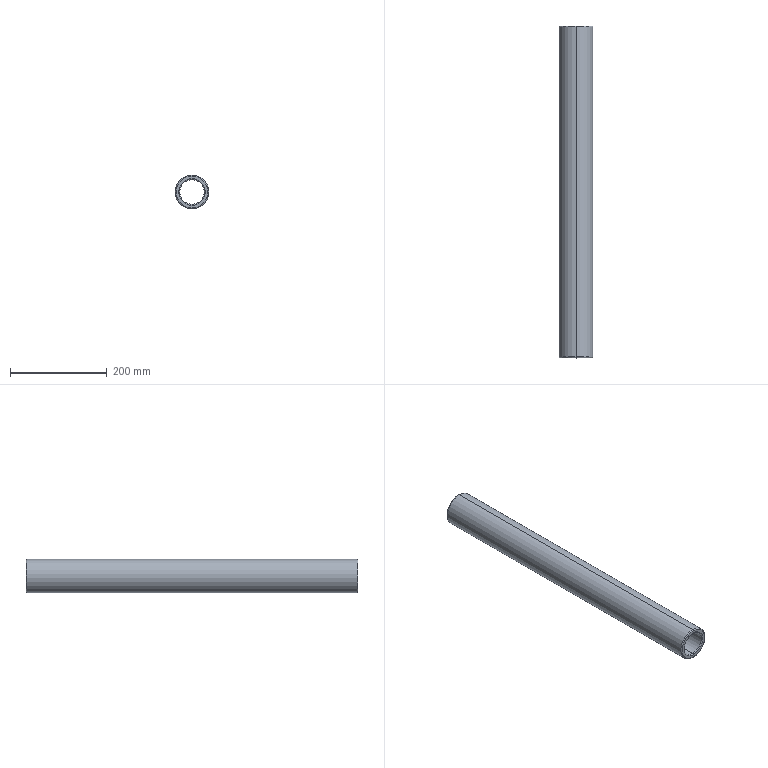Part | SolidWorks | features MBimport 1 | 1 solid | 14 faces | box 70 x 687.27 x 70 mm | volume 1240304 mm3 | torus 8 | cylinder 4 | plane 2 | commonest cylinder face diameters 51 x2 70 x2
STEP:
#1=CARTESIAN_POINT('',(0.,-685.27,35.));
#2=VERTEX_POINT('',#1);
#3=CARTESIAN_POINT('',(0.,-685.27,-35.));
#4=VERTEX_POINT('',#3);
#5=CARTESIAN_POINT('',(0.,-685.27,0.));
#6=DIRECTION('',(0.,1.,0.));
#7=DIRECTION('',(0.,0.,-1.));
#8=AXIS2_PLACEMENT_3D('',#5,#6,#7);
#9=CIRCLE('',#8,35.);
#10=EDGE_CURVE('',#2,#4,#9,.T.);
#11=ORIENTED_EDGE('',*,*,#10,.F.);
#12=CARTESIAN_POINT('',(0.,-687.27,33.));
#13=VERTEX_POINT('',#12);
#14=CARTESIAN_POINT('',(0.,-685.27,33.));
#15=DIRECTION('',(1.,0.,0.));
#16=DIRECTION('',(0.,0.,-1.));
#17=AXIS2_PLACEMENT_3D('',#14,#15,#16);
#18=CIRCLE('',#17,2.);
#19=EDGE_CURVE('',#2,#13,#18,.T.);
#20=ORIENTED_EDGE('',*,*,#19,.T.);
#21=CARTESIAN_POINT('',(0.,-687.27,-33.));
#22=VERTEX_POINT('',#21);
#23=CARTESIAN_POINT('',(0.,-687.27,0.));
#24=DIRECTION('',(0.,-1.,0.));
#25=DIRECTION('',(0.,0.,-1.));
#26=AXIS2_PLACEMENT_3D('',#23,#24,#25);
#27=CIRCLE('',#26,33.);
#28=EDGE_CURVE('',#22,#13,#27,.T.);
#29=ORIENTED_EDGE('',*,*,#28,.F.);
#30=CARTESIAN_POINT('',(0.,-685.27,-33.));
#31=DIRECTION('',(-1.,0.,0.));
#32=DIRECTION('',(0.,0.,1.));
#33=AXIS2_PLACEMENT_3D('',#30,#31,#32);
#34=CIRCLE('',#33,2.);
#35=EDGE_CURVE('',#4,#22,#34,.T.);
#36=ORIENTED_EDGE('',*,*,#35,.F.);
#37=EDGE_LOOP('',(#11,#20,#29,#36));
#38=FACE_OUTER_BOUND('',#37,.T.);
#39=CARTESIAN_POINT('',(0.,-685.27,0.));
#40=DIRECTION('',(0.,-1.,0.));
#41=DIRECTION('',(0.,0.,-1.));
#42=AXIS2_PLACEMENT_3D('',#39,#40,#41);
#43=TOROIDAL_SURFACE('',#42,33.,2.);
#44=ADVANCED_FACE('',(#38),#43,.T.);
#45=CARTESIAN_POINT('',(0.,0.,33.));
#46=VERTEX_POINT('',#45);
#47=CARTESIAN_POINT('',(0.,0.,-33.));
#48=VERTEX_POINT('',#47);
#49=CARTESIAN_POINT('',(0.,0.,0.));
#50=DIRECTION('',(0.,1.,0.));
#51=DIRECTION('',(0.,0.,-1.));
#52=AXIS2_PLACEMENT_3D('',#49,#50,#51);
#53=CIRCLE('',#52,33.);
#54=EDGE_CURVE('',#46,#48,#53,.T.);
#55=ORIENTED_EDGE('',*,*,#54,.F.);
#56=CARTESIAN_POINT('',(0.,-2.,35.));
#57=VERTEX_POINT('',#56);
#58=CARTESIAN_POINT('',(0.,-2.,33.));
#59=DIRECTION('',(1.,0.,0.));
#60=DIRECTION('',(0.,0.,-1.));
#61=AXIS2_PLACEMENT_3D('',#58,#59,#60);
#62=CIRCLE('',#61,2.);
#63=EDGE_CURVE('',#46,#57,#62,.T.);
#64=ORIENTED_EDGE('',*,*,#63,.T.);
#65=CARTESIAN_POINT('',(0.,-2.,-35.));
#66=VERTEX_POINT('',#65);
#67=CARTESIAN_POINT('',(0.,-2.,0.));
#68=DIRECTION('',(0.,-1.,0.));
#69=DIRECTION('',(0.,0.,-1.));
#70=AXIS2_PLACEMENT_3D('',#67,#68,#69);
#71=CIRCLE('',#70,35.);
#72=EDGE_CURVE('',#66,#57,#71,.T.);
#73=ORIENTED_EDGE('',*,*,#72,.F.);
#74=CARTESIAN_POINT('',(0.,-2.,-33.));
#75=DIRECTION('',(-1.,0.,0.));
#76=DIRECTION('',(0.,0.,1.));
#77=AXIS2_PLACEMENT_3D('',#74,#75,#76);
#78=CIRCLE('',#77,2.);
#79=EDGE_CURVE('',#48,#66,#78,.T.);
#80=ORIENTED_EDGE('',*,*,#79,.F.);
#81=EDGE_LOOP('',(#55,#64,#73,#80));
#82=FACE_OUTER_BOUND('',#81,.T.);
#83=CARTESIAN_POINT('',(0.,-2.,0.));
#84=DIRECTION('',(0.,-1.,0.));
#85=DIRECTION('',(0.,0.,-1.));
#86=AXIS2_PLACEMENT_3D('',#83,#84,#85);
#87=TOROIDAL_SURFACE('',#86,33.,2.);
#88=ADVANCED_FACE('',(#82),#87,.T.);
#89=CARTESIAN_POINT('',(0.,-2.,25.5));
#90=VERTEX_POINT('',#89);
#91=CARTESIAN_POINT('',(0.,-2.,-25.5));
#92=VERTEX_POINT('',#91);
#93=CARTESIAN_POINT('',(0.,-2.,0.));
#94=DIRECTION('',(0.,1.,0.));
#95=DIRECTION('',(0.,0.,-1.));
#96=AXIS2_PLACEMENT_3D('',#93,#94,#95);
#97=CIRCLE('',#96,25.5);
#98=EDGE_CURVE('',#90,#92,#97,.T.);
#99=ORIENTED_EDGE('',*,*,#98,.F.);
#100=CARTESIAN_POINT('',(0.,0.,27.5));
#101=VERTEX_POINT('',#100);
#102=CARTESIAN_POINT('',(0.,-2.,27.5));
#103=DIRECTION('',(1.,0.,0.));
#104=DIRECTION('',(0.,0.,-1.));
#105=AXIS2_PLACEMENT_3D('',#102,#103,#104);
#106=CIRCLE('',#105,2.);
#107=EDGE_CURVE('',#90,#101,#106,.T.);
#108=ORIENTED_EDGE('',*,*,#107,.T.);
#109=CARTESIAN_POINT('',(0.,0.,-27.5));
#110=VERTEX_POINT('',#109);
#111=CARTESIAN_POINT('',(0.,0.,0.));
#112=DIRECTION('',(0.,-1.,0.));
#113=DIRECTION('',(0.,0.,-1.));
#114=AXIS2_PLACEMENT_3D('',#111,#112,#113);
#115=CIRCLE('',#114,27.5);
#116=EDGE_CURVE('',#110,#101,#115,.T.);
#117=ORIENTED_EDGE('',*,*,#116,.F.);
#118=CARTESIAN_POINT('',(0.,-2.,-27.5));
#119=DIRECTION('',(-1.,0.,0.));
#120=DIRECTION('',(0.,0.,1.));
#121=AXIS2_PLACEMENT_3D('',#118,#119,#120);
#122=CIRCLE('',#121,2.);
#123=EDGE_CURVE('',#92,#110,#122,.T.);
#124=ORIENTED_EDGE('',*,*,#123,.F.);
#125=EDGE_LOOP('',(#99,#108,#117,#124));
#126=FACE_OUTER_BOUND('',#125,.T.);
#127=CARTESIAN_POINT('',(0.,-2.,0.));
#128=DIRECTION('',(0.,-1.,0.));
#129=DIRECTION('',(0.,0.,-1.));
#130=AXIS2_PLACEMENT_3D('',#127,#128,#129);
#131=TOROIDAL_SURFACE('',#130,27.5,2.);
#132=ADVANCED_FACE('',(#126),#131,.T.);
#133=CARTESIAN_POINT('',(0.,-687.27,27.5));
#134=VERTEX_POINT('',#133);
#135=CARTESIAN_POINT('',(0.,-687.27,-27.5));
#136=VERTEX_POINT('',#135);
#137=CARTESIAN_POINT('',(0.,-687.27,0.));
#138=DIRECTION('',(0.,1.,0.));
#139=DIRECTION('',(0.,0.,-1.));
#140=AXIS2_PLACEMENT_3D('',#137,#138,#139);
#141=CIRCLE('',#140,27.5);
#142=EDGE_CURVE('',#134,#136,#141,.T.);
#143=ORIENTED_EDGE('',*,*,#142,.F.);
#144=CARTESIAN_POINT('',(0.,-685.27,25.5));
#145=VERTEX_POINT('',#144);
#146=CARTESIAN_POINT('',(0.,-685.27,27.5));
#147=DIRECTION('',(1.,0.,0.));
#148=DIRECTION('',(0.,0.,-1.));
#149=AXIS2_PLACEMENT_3D('',#146,#147,#148);
#150=CIRCLE('',#149,2.);
#151=EDGE_CURVE('',#134,#145,#150,.T.);
#152=ORIENTED_EDGE('',*,*,#151,.T.);
#153=CARTESIAN_POINT('',(0.,-685.27,-25.5));
#154=VERTEX_POINT('',#153);
#155=CARTESIAN_POINT('',(0.,-685.27,0.));
#156=DIRECTION('',(0.,-1.,0.));
#157=DIRECTION('',(0.,0.,-1.));
#158=AXIS2_PLACEMENT_3D('',#155,#156,#157);
#159=CIRCLE('',#158,25.5);
#160=EDGE_CURVE('',#154,#145,#159,.T.);
#161=ORIENTED_EDGE('',*,*,#160,.F.);
#162=CARTESIAN_POINT('',(0.,-685.27,-27.5));
#163=DIRECTION('',(-1.,0.,0.));
#164=DIRECTION('',(0.,0.,1.));
#165=AXIS2_PLACEMENT_3D('',#162,#163,#164);
#166=CIRCLE('',#165,2.);
#167=EDGE_CURVE('',#136,#154,#166,.T.);
#168=ORIENTED_EDGE('',*,*,#167,.F.);
#169=EDGE_LOOP('',(#143,#152,#161,#168));
#170=FACE_OUTER_BOUND('',#169,.T.);
#171=CARTESIAN_POINT('',(0.,-685.27,0.));
#172=DIRECTION('',(0.,-1.,0.));
#173=DIRECTION('',(0.,0.,-1.));
#174=AXIS2_PLACEMENT_3D('',#171,#172,#173);
#175=TOROIDAL_SURFACE('',#174,27.5,2.);
#176=ADVANCED_FACE('',(#170),#175,.T.);
#177=CARTESIAN_POINT('',(0.,-685.27,0.));
#178=DIRECTION('',(0.,-1.,0.));
#179=DIRECTION('',(0.,0.,-1.));
#180=AXIS2_PLACEMENT_3D('',#177,#178,#179);
#181=CIRCLE('',#180,25.5);
#182=EDGE_CURVE('',#145,#154,#181,.T.);
#183=ORIENTED_EDGE('',*,*,#182,.T.);
#184=CARTESIAN_POINT('',(0.,-687.27,-25.5));
#185=DIRECTION('',(0.,1.,0.));
#186=VECTOR('',#185,1000.);
#187=LINE('',#184,#186);
#188=EDGE_CURVE('',#154,#92,#187,.T.);
#189=ORIENTED_EDGE('',*,*,#188,.T.);
#190=CARTESIAN_POINT('',(0.,-2.,0.));
#191=DIRECTION('',(0.,1.,0.));
#192=DIRECTION('',(0.,0.,-1.));
#193=AXIS2_PLACEMENT_3D('',#190,#191,#192);
#194=CIRCLE('',#193,25.5);
#195=EDGE_CURVE('',#92,#90,#194,.T.);
#196=ORIENTED_EDGE('',*,*,#195,.T.);
#197=CARTESIAN_POINT('',(0.,-687.27,25.5));
#198=DIRECTION('',(0.,1.,0.));
#199=VECTOR('',#198,1000.);
#200=LINE('',#197,#199);
#201=EDGE_CURVE('',#145,#90,#200,.T.);
#202=ORIENTED_EDGE('',*,*,#201,.F.);
#203=EDGE_LOOP('',(#183,#189,#196,#202));
#204=FACE_OUTER_BOUND('',#203,.T.);
#205=CARTESIAN_POINT('',(0.,-687.27,0.));
#206=DIRECTION('',(0.,1.,0.));
#207=DIRECTION('',(0.,0.,1.));
#208=AXIS2_PLACEMENT_3D('',#205,#206,#207);
#209=CYLINDRICAL_SURFACE('',#208,25.5);
#210=ADVANCED_FACE('',(#204),#209,.F.);
#211=ORIENTED_EDGE('',*,*,#10,.T.);
#212=CARTESIAN_POINT('',(0.,-687.27,-35.));
#213=DIRECTION('',(0.,1.,0.));
#214=VECTOR('',#213,1000.);
#215=LINE('',#212,#214);
#216=EDGE_CURVE('',#4,#66,#215,.T.);
#217=ORIENTED_EDGE('',*,*,#216,.T.);
#218=ORIENTED_EDGE('',*,*,#72,.T.);
#219=CARTESIAN_POINT('',(0.,-687.27,35.));
#220=DIRECTION('',(0.,1.,0.));
#221=VECTOR('',#220,1000.);
#222=LINE('',#219,#221);
#223=EDGE_CURVE('',#2,#57,#222,.T.);
#224=ORIENTED_EDGE('',*,*,#223,.F.);
#225=EDGE_LOOP('',(#211,#217,#218,#224));
#226=FACE_OUTER_BOUND('',#225,.T.);
#227=CARTESIAN_POINT('',(0.,-687.27,0.));
#228=DIRECTION('',(0.,1.,0.));
#229=DIRECTION('',(0.,0.,1.));
#230=AXIS2_PLACEMENT_3D('',#227,#228,#229);
#231=CYLINDRICAL_SURFACE('',#230,35.);
#232=ADVANCED_FACE('',(#226),#231,.T.);
#233=ORIENTED_EDGE('',*,*,#216,.F.);
#234=CARTESIAN_POINT('',(0.,-685.27,0.));
#235=DIRECTION('',(0.,1.,0.));
#236=DIRECTION('',(0.,0.,-1.));
#237=AXIS2_PLACEMENT_3D('',#234,#235,#236);
#238=CIRCLE('',#237,35.);
#239=EDGE_CURVE('',#4,#2,#238,.T.);
#240=ORIENTED_EDGE('',*,*,#239,.T.);
#241=ORIENTED_EDGE('',*,*,#223,.T.);
#242=CARTESIAN_POINT('',(0.,-2.,0.));
#243=DIRECTION('',(0.,-1.,0.));
#244=DIRECTION('',(0.,0.,-1.));
#245=AXIS2_PLACEMENT_3D('',#242,#243,#244);
#246=CIRCLE('',#245,35.);
#247=EDGE_CURVE('',#57,#66,#246,.T.);
#248=ORIENTED_EDGE('',*,*,#247,.T.);
#249=EDGE_LOOP('',(#233,#240,#241,#248));
#250=FACE_OUTER_BOUND('',#249,.T.);
#251=CARTESIAN_POINT('',(0.,-687.27,0.));
#252=DIRECTION('',(0.,1.,0.));
#253=DIRECTION('',(0.,0.,1.));
#254=AXIS2_PLACEMENT_3D('',#251,#252,#253);
#255=CYLINDRICAL_SURFACE('',#254,35.);
#256=ADVANCED_FACE('',(#250),#255,.T.);
#257=ORIENTED_EDGE('',*,*,#188,.F.);
#258=ORIENTED_EDGE('',*,*,#160,.T.);
#259=ORIENTED_EDGE('',*,*,#201,.T.);
#260=ORIENTED_EDGE('',*,*,#98,.T.);
#261=EDGE_LOOP('',(#257,#258,#259,#260));
#262=FACE_OUTER_BOUND('',#261,.T.);
#263=CARTESIAN_POINT('',(0.,-687.27,0.));
#264=DIRECTION('',(0.,1.,0.));
#265=DIRECTION('',(0.,0.,1.));
#266=AXIS2_PLACEMENT_3D('',#263,#264,#265);
#267=CYLINDRICAL_SURFACE('',#266,25.5);
#268=ADVANCED_FACE('',(#262),#267,.F.);
#269=ORIENTED_EDGE('',*,*,#28,.T.);
#270=CARTESIAN_POINT('',(0.,-687.27,0.));
#271=DIRECTION('',(0.,-1.,0.));
#272=DIRECTION('',(0.,0.,-1.));
#273=AXIS2_PLACEMENT_3D('',#270,#271,#272);
#274=CIRCLE('',#273,33.);
#275=EDGE_CURVE('',#13,#22,#274,.T.);
#276=ORIENTED_EDGE('',*,*,#275,.T.);
#277=EDGE_LOOP('',(#269,#276));
#278=FACE_OUTER_BOUND('',#277,.T.);
#279=CARTESIAN_POINT('',(0.,-687.27,0.));
#280=DIRECTION('',(0.,1.,0.));
#281=DIRECTION('',(0.,0.,-1.));
#282=AXIS2_PLACEMENT_3D('',#279,#280,#281);
#283=CIRCLE('',#282,27.5);
#284=EDGE_CURVE('',#136,#134,#283,.T.);
#285=ORIENTED_EDGE('',*,*,#284,.T.);
#286=ORIENTED_EDGE('',*,*,#142,.T.);
#287=EDGE_LOOP('',(#285,#286));
#288=FACE_BOUND('',#287,.T.);
#289=CARTESIAN_POINT('',(0.,-687.27,0.));
#290=DIRECTION('',(0.,-1.,0.));
#291=DIRECTION('',(0.,0.,-1.));
#292=AXIS2_PLACEMENT_3D('',#289,#290,#291);
#293=PLANE('',#292);
#294=ADVANCED_FACE('',(#278,#288),#293,.T.);
#295=ORIENTED_EDGE('',*,*,#116,.T.);
#296=CARTESIAN_POINT('',(0.,0.,0.));
#297=DIRECTION('',(0.,-1.,0.));
#298=DIRECTION('',(0.,0.,-1.));
#299=AXIS2_PLACEMENT_3D('',#296,#297,#298);
#300=CIRCLE('',#299,27.5);
#301=EDGE_CURVE('',#101,#110,#300,.T.);
#302=ORIENTED_EDGE('',*,*,#301,.T.);
#303=EDGE_LOOP('',(#295,#302));
#304=FACE_BOUND('',#303,.T.);
#305=CARTESIAN_POINT('',(0.,0.,0.));
#306=DIRECTION('',(0.,1.,0.));
#307=DIRECTION('',(0.,0.,-1.));
#308=AXIS2_PLACEMENT_3D('',#305,#306,#307);
#309=CIRCLE('',#308,33.);
#310=EDGE_CURVE('',#48,#46,#309,.T.);
#311=ORIENTED_EDGE('',*,*,#310,.T.);
#312=ORIENTED_EDGE('',*,*,#54,.T.);
#313=EDGE_LOOP('',(#311,#312));
#314=FACE_OUTER_BOUND('',#313,.T.);
#315=CARTESIAN_POINT('',(0.,0.,0.));
#316=DIRECTION('',(0.,-1.,0.));
#317=DIRECTION('',(0.,0.,-1.));
#318=AXIS2_PLACEMENT_3D('',#315,#316,#317);
#319=PLANE('',#318);
#320=ADVANCED_FACE('',(#304,#314),#319,.F.);
#321=ORIENTED_EDGE('',*,*,#151,.F.);
#322=ORIENTED_EDGE('',*,*,#284,.F.);
#323=ORIENTED_EDGE('',*,*,#167,.T.);
#324=ORIENTED_EDGE('',*,*,#182,.F.);
#325=EDGE_LOOP('',(#321,#322,#323,#324));
#326=FACE_OUTER_BOUND('',#325,.T.);
#327=CARTESIAN_POINT('',(0.,-685.27,0.));
#328=DIRECTION('',(0.,-1.,0.));
#329=DIRECTION('',(0.,0.,-1.));
#330=AXIS2_PLACEMENT_3D('',#327,#328,#329);
#331=TOROIDAL_SURFACE('',#330,27.5,2.);
#332=ADVANCED_FACE('',(#326),#331,.T.);
#333=ORIENTED_EDGE('',*,*,#107,.F.);
#334=ORIENTED_EDGE('',*,*,#195,.F.);
#335=ORIENTED_EDGE('',*,*,#123,.T.);
#336=ORIENTED_EDGE('',*,*,#301,.F.);
#337=EDGE_LOOP('',(#333,#334,#335,#336));
#338=FACE_OUTER_BOUND('',#337,.T.);
#339=CARTESIAN_POINT('',(0.,-2.,0.));
#340=DIRECTION('',(0.,-1.,0.));
#341=DIRECTION('',(0.,0.,-1.));
#342=AXIS2_PLACEMENT_3D('',#339,#340,#341);
#343=TOROIDAL_SURFACE('',#342,27.5,2.);
#344=ADVANCED_FACE('',(#338),#343,.T.);
#345=ORIENTED_EDGE('',*,*,#63,.F.);
#346=ORIENTED_EDGE('',*,*,#310,.F.);
#347=ORIENTED_EDGE('',*,*,#79,.T.);
#348=ORIENTED_EDGE('',*,*,#247,.F.);
#349=EDGE_LOOP('',(#345,#346,#347,#348));
#350=FACE_OUTER_BOUND('',#349,.T.);
#351=CARTESIAN_POINT('',(0.,-2.,0.));
#352=DIRECTION('',(0.,-1.,0.));
#353=DIRECTION('',(0.,0.,-1.));
#354=AXIS2_PLACEMENT_3D('',#351,#352,#353);
#355=TOROIDAL_SURFACE('',#354,33.,2.);
#356=ADVANCED_FACE('',(#350),#355,.T.);
#357=ORIENTED_EDGE('',*,*,#19,.F.);
#358=ORIENTED_EDGE('',*,*,#239,.F.);
#359=ORIENTED_EDGE('',*,*,#35,.T.);
#360=ORIENTED_EDGE('',*,*,#275,.F.);
#361=EDGE_LOOP('',(#357,#358,#359,#360));
#362=FACE_OUTER_BOUND('',#361,.T.);
#363=CARTESIAN_POINT('',(0.,-685.27,0.));
#364=DIRECTION('',(0.,-1.,0.));
#365=DIRECTION('',(0.,0.,-1.));
#366=AXIS2_PLACEMENT_3D('',#363,#364,#365);
#367=TOROIDAL_SURFACE('',#366,33.,2.);
#368=ADVANCED_FACE('',(#362),#367,.T.);
#369=CLOSED_SHELL('',(#44,#88,#132,#176,#210,#232,#256,#268,#294,#320,#332,#344,#356,#368));
#370=MANIFOLD_SOLID_BREP('',#369);
#371=CARTESIAN_POINT('',(0.,0.,0.));
#372=DIRECTION('',(0.,0.,1.));
#373=DIRECTION('',(1.,0.,0.));
#374=AXIS2_PLACEMENT_3D('',#371,#372,#373);
#375=(LENGTH_UNIT()NAMED_UNIT(*)SI_UNIT(.MILLI.,.METRE.));
#376=UNCERTAINTY_MEASURE_WITH_UNIT(LENGTH_MEASURE(0.00001),#375,'','');
#377=(NAMED_UNIT(*)PLANE_ANGLE_UNIT()SI_UNIT($,.RADIAN.));
#378=(NAMED_UNIT(*)SI_UNIT($,.STERADIAN.)SOLID_ANGLE_UNIT());
#379=(GEOMETRIC_REPRESENTATION_CONTEXT(3)GLOBAL_UNCERTAINTY_ASSIGNED_CONTEXT((#376))GLOBAL_UNIT_ASSIGNED_CONTEXT((#375,#377,#378))REPRESENTATION_CONTEXT('',''));
#380=ADVANCED_BREP_SHAPE_REPRESENTATION('',(#370,#374),#379);